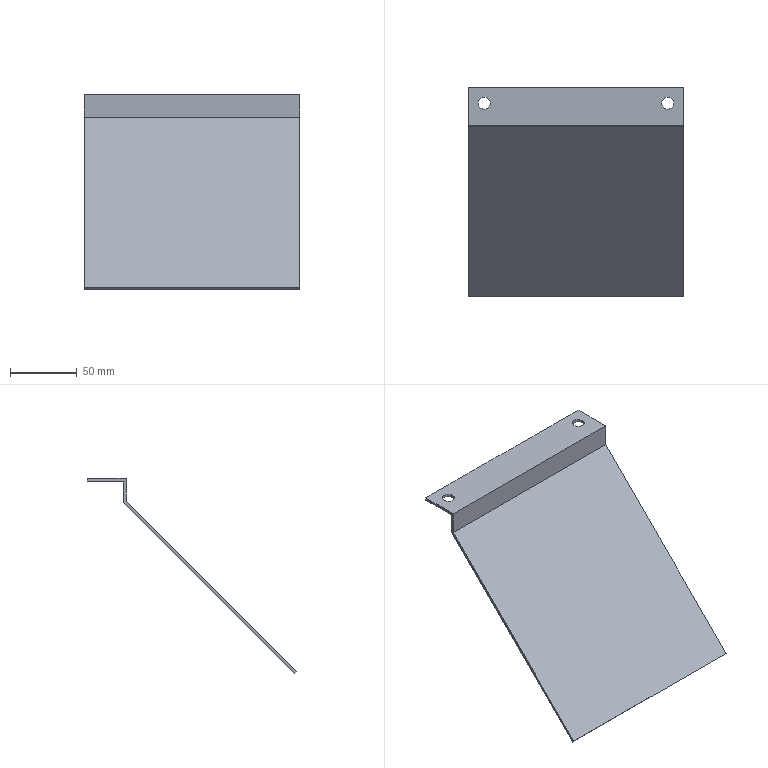Part | STEP file | lll_id4358_x_t | 1 solid | 12 faces | box 161.869 x 157.279 x 146.693 mm | volume 73016 mm3 | plane 10 | cylinder 2 | commonest cylinder face diameters 9 x2
STEP:
#1=CARTESIAN_POINT('',(1255.459,232.307,-325.279));
#2=VERTEX_POINT('',#1);
#3=CARTESIAN_POINT('',(1255.459,233.721,-326.693));
#4=VERTEX_POINT('',#3);
#5=CARTESIAN_POINT('',(1255.459,232.307,-325.279));
#6=DIRECTION('',(0.,0.7071,-0.7071));
#7=VECTOR('',#6,1.);
#8=LINE('',#5,#7);
#9=EDGE_CURVE('',#2,#4,#8,.T.);
#10=ORIENTED_EDGE('',*,*,#9,.T.);
#11=CARTESIAN_POINT('',(1417.328,233.721,-326.693));
#12=VERTEX_POINT('',#11);
#13=CARTESIAN_POINT('',(1417.328,233.721,-326.693));
#14=DIRECTION('',(-1.,0.,0.));
#15=VECTOR('',#14,1.);
#16=LINE('',#13,#15);
#17=EDGE_CURVE('',#12,#4,#16,.T.);
#18=ORIENTED_EDGE('',*,*,#17,.F.);
#19=CARTESIAN_POINT('',(1417.328,232.307,-325.279));
#20=VERTEX_POINT('',#19);
#21=CARTESIAN_POINT('',(1417.328,232.307,-325.279));
#22=DIRECTION('',(0.,0.7071,-0.7071));
#23=VECTOR('',#22,1.);
#24=LINE('',#21,#23);
#25=EDGE_CURVE('',#20,#12,#24,.T.);
#26=ORIENTED_EDGE('',*,*,#25,.F.);
#27=CARTESIAN_POINT('',(1417.328,232.307,-325.279));
#28=DIRECTION('',(-1.,0.,0.));
#29=VECTOR('',#28,1.);
#30=LINE('',#27,#29);
#31=EDGE_CURVE('',#20,#2,#30,.T.);
#32=ORIENTED_EDGE('',*,*,#31,.T.);
#33=EDGE_LOOP('',(#10,#18,#26,#32));
#34=FACE_OUTER_BOUND('',#33,.T.);
#35=CARTESIAN_POINT('',(1417.328,232.307,-325.279));
#36=DIRECTION('',(0.,-0.7071,-0.7071));
#37=DIRECTION('',(-1.,0.,0.));
#38=AXIS2_PLACEMENT_3D('',#35,#36,#37);
#39=PLANE('',#38);
#40=ADVANCED_FACE('',(#34),#39,.T.);
#41=CARTESIAN_POINT('',(1417.328,360.382,-197.204));
#42=VERTEX_POINT('',#41);
#43=CARTESIAN_POINT('',(1417.328,246.449,-311.137));
#44=DIRECTION('',(0.,-0.7071,-0.7071));
#45=VECTOR('',#44,1.);
#46=LINE('',#43,#45);
#47=EDGE_CURVE('',#42,#20,#46,.T.);
#48=ORIENTED_EDGE('',*,*,#47,.T.);
#49=ORIENTED_EDGE('',*,*,#25,.T.);
#50=CARTESIAN_POINT('',(1417.328,362.38,-198.034));
#51=VERTEX_POINT('',#50);
#52=CARTESIAN_POINT('',(1417.328,247.863,-312.551));
#53=DIRECTION('',(0.,-0.7071,-0.7071));
#54=VECTOR('',#53,1.);
#55=LINE('',#52,#54);
#56=EDGE_CURVE('',#51,#12,#55,.T.);
#57=ORIENTED_EDGE('',*,*,#56,.F.);
#58=CARTESIAN_POINT('',(1417.328,362.414,-182.));
#59=VERTEX_POINT('',#58);
#60=CARTESIAN_POINT('',(1417.328,362.414,-182.004));
#61=DIRECTION('',(0.,-0.00212,-1.));
#62=VECTOR('',#61,1.);
#63=LINE('',#60,#62);
#64=EDGE_CURVE('',#59,#51,#63,.T.);
#65=ORIENTED_EDGE('',*,*,#64,.F.);
#66=CARTESIAN_POINT('',(1417.328,389.586,-182.));
#67=VERTEX_POINT('',#66);
#68=CARTESIAN_POINT('',(1417.328,359.586,-182.));
#69=DIRECTION('',(0.,1.,0.));
#70=VECTOR('',#69,1.);
#71=LINE('',#68,#70);
#72=EDGE_CURVE('',#59,#67,#71,.T.);
#73=ORIENTED_EDGE('',*,*,#72,.T.);
#74=CARTESIAN_POINT('',(1417.328,389.586,-180.));
#75=VERTEX_POINT('',#74);
#76=CARTESIAN_POINT('',(1417.328,389.586,-293.137));
#77=DIRECTION('',(0.,0.,-1.));
#78=VECTOR('',#77,1.);
#79=LINE('',#76,#78);
#80=EDGE_CURVE('',#75,#67,#79,.T.);
#81=ORIENTED_EDGE('',*,*,#80,.F.);
#82=CARTESIAN_POINT('',(1417.328,360.418,-180.));
#83=VERTEX_POINT('',#82);
#84=CARTESIAN_POINT('',(1417.328,359.586,-180.));
#85=DIRECTION('',(0.,1.,0.));
#86=VECTOR('',#85,1.);
#87=LINE('',#84,#86);
#88=EDGE_CURVE('',#83,#75,#87,.T.);
#89=ORIENTED_EDGE('',*,*,#88,.F.);
#90=CARTESIAN_POINT('',(1417.328,360.178,-293.378));
#91=DIRECTION('',(0.,-0.00212,-1.));
#92=VECTOR('',#91,1.);
#93=LINE('',#90,#92);
#94=EDGE_CURVE('',#83,#42,#93,.T.);
#95=ORIENTED_EDGE('',*,*,#94,.T.);
#96=EDGE_LOOP('',(#48,#49,#57,#65,#73,#81,#89,#95));
#97=FACE_OUTER_BOUND('',#96,.T.);
#98=CARTESIAN_POINT('',(1417.328,246.449,-311.137));
#99=DIRECTION('',(-1.,0.,0.));
#100=DIRECTION('',(0.,0.7071,0.7071));
#101=AXIS2_PLACEMENT_3D('',#98,#99,#100);
#102=PLANE('',#101);
#103=ADVANCED_FACE('',(#97),#102,.F.);
#104=CARTESIAN_POINT('',(1255.459,362.38,-198.034));
#105=VERTEX_POINT('',#104);
#106=CARTESIAN_POINT('',(1255.459,247.863,-312.551));
#107=DIRECTION('',(0.,0.7071,0.7071));
#108=VECTOR('',#107,1.);
#109=LINE('',#106,#108);
#110=EDGE_CURVE('',#4,#105,#109,.T.);
#111=ORIENTED_EDGE('',*,*,#110,.F.);
#112=ORIENTED_EDGE('',*,*,#9,.F.);
#113=CARTESIAN_POINT('',(1255.459,360.382,-197.204));
#114=VERTEX_POINT('',#113);
#115=CARTESIAN_POINT('',(1255.459,246.449,-311.137));
#116=DIRECTION('',(0.,0.7071,0.7071));
#117=VECTOR('',#116,1.);
#118=LINE('',#115,#117);
#119=EDGE_CURVE('',#2,#114,#118,.T.);
#120=ORIENTED_EDGE('',*,*,#119,.T.);
#121=CARTESIAN_POINT('',(1255.459,360.418,-180.));
#122=VERTEX_POINT('',#121);
#123=CARTESIAN_POINT('',(1255.459,360.178,-293.378));
#124=DIRECTION('',(0.,-0.00212,-1.));
#125=VECTOR('',#124,1.);
#126=LINE('',#123,#125);
#127=EDGE_CURVE('',#122,#114,#126,.T.);
#128=ORIENTED_EDGE('',*,*,#127,.F.);
#129=CARTESIAN_POINT('',(1255.459,389.586,-180.));
#130=VERTEX_POINT('',#129);
#131=CARTESIAN_POINT('',(1255.459,359.586,-180.));
#132=DIRECTION('',(0.,-1.,0.));
#133=VECTOR('',#132,1.);
#134=LINE('',#131,#133);
#135=EDGE_CURVE('',#130,#122,#134,.T.);
#136=ORIENTED_EDGE('',*,*,#135,.F.);
#137=CARTESIAN_POINT('',(1255.459,389.586,-182.));
#138=VERTEX_POINT('',#137);
#139=CARTESIAN_POINT('',(1255.459,389.586,-180.));
#140=DIRECTION('',(0.,0.,-1.));
#141=VECTOR('',#140,1.);
#142=LINE('',#139,#141);
#143=EDGE_CURVE('',#130,#138,#142,.T.);
#144=ORIENTED_EDGE('',*,*,#143,.T.);
#145=CARTESIAN_POINT('',(1255.459,362.414,-182.));
#146=VERTEX_POINT('',#145);
#147=CARTESIAN_POINT('',(1255.459,359.586,-182.));
#148=DIRECTION('',(0.,-1.,0.));
#149=VECTOR('',#148,1.);
#150=LINE('',#147,#149);
#151=EDGE_CURVE('',#138,#146,#150,.T.);
#152=ORIENTED_EDGE('',*,*,#151,.T.);
#153=CARTESIAN_POINT('',(1255.459,362.414,-182.004));
#154=DIRECTION('',(0.,-0.00212,-1.));
#155=VECTOR('',#154,1.);
#156=LINE('',#153,#155);
#157=EDGE_CURVE('',#146,#105,#156,.T.);
#158=ORIENTED_EDGE('',*,*,#157,.T.);
#159=EDGE_LOOP('',(#111,#112,#120,#128,#136,#144,#152,#158));
#160=FACE_OUTER_BOUND('',#159,.T.);
#161=CARTESIAN_POINT('',(1255.459,246.449,-311.137));
#162=DIRECTION('',(-1.,0.,0.));
#163=DIRECTION('',(0.,0.7071,0.7071));
#164=AXIS2_PLACEMENT_3D('',#161,#162,#163);
#165=PLANE('',#164);
#166=ADVANCED_FACE('',(#160),#165,.T.);
#167=ORIENTED_EDGE('',*,*,#56,.T.);
#168=ORIENTED_EDGE('',*,*,#17,.T.);
#169=ORIENTED_EDGE('',*,*,#110,.T.);
#170=CARTESIAN_POINT('',(-1607.432,362.38,-198.034));
#171=DIRECTION('',(-1.,0.,0.));
#172=VECTOR('',#171,1.);
#173=LINE('',#170,#172);
#174=EDGE_CURVE('',#51,#105,#173,.T.);
#175=ORIENTED_EDGE('',*,*,#174,.F.);
#176=EDGE_LOOP('',(#167,#168,#169,#175));
#177=FACE_OUTER_BOUND('',#176,.T.);
#178=CARTESIAN_POINT('',(1417.328,247.863,-312.551));
#179=DIRECTION('',(0.,-0.7071,0.7071));
#180=DIRECTION('',(0.,0.7071,0.7071));
#181=AXIS2_PLACEMENT_3D('',#178,#179,#180);
#182=PLANE('',#181);
#183=ADVANCED_FACE('',(#177),#182,.F.);
#184=CARTESIAN_POINT('',(1417.328,360.382,-197.204));
#185=DIRECTION('',(-1.,0.,0.));
#186=VECTOR('',#185,1.);
#187=LINE('',#184,#186);
#188=EDGE_CURVE('',#42,#114,#187,.T.);
#189=ORIENTED_EDGE('',*,*,#188,.T.);
#190=ORIENTED_EDGE('',*,*,#119,.F.);
#191=ORIENTED_EDGE('',*,*,#31,.F.);
#192=ORIENTED_EDGE('',*,*,#47,.F.);
#193=EDGE_LOOP('',(#189,#190,#191,#192));
#194=FACE_OUTER_BOUND('',#193,.T.);
#195=CARTESIAN_POINT('',(1417.328,246.449,-311.137));
#196=DIRECTION('',(0.,-0.7071,0.7071));
#197=DIRECTION('',(0.,0.7071,0.7071));
#198=AXIS2_PLACEMENT_3D('',#195,#196,#197);
#199=PLANE('',#198);
#200=ADVANCED_FACE('',(#194),#199,.T.);
#201=ORIENTED_EDGE('',*,*,#64,.T.);
#202=ORIENTED_EDGE('',*,*,#174,.T.);
#203=ORIENTED_EDGE('',*,*,#157,.F.);
#204=CARTESIAN_POINT('',(-1607.432,362.414,-182.));
#205=DIRECTION('',(-1.,0.,0.));
#206=VECTOR('',#205,1.);
#207=LINE('',#204,#206);
#208=EDGE_CURVE('',#59,#146,#207,.T.);
#209=ORIENTED_EDGE('',*,*,#208,.F.);
#210=EDGE_LOOP('',(#201,#202,#203,#209));
#211=FACE_OUTER_BOUND('',#210,.T.);
#212=CARTESIAN_POINT('',(-1607.432,362.414,-182.004));
#213=DIRECTION('',(0.,-1.,0.00212));
#214=DIRECTION('',(0.,0.00212,1.));
#215=AXIS2_PLACEMENT_3D('',#212,#213,#214);
#216=PLANE('',#215);
#217=ADVANCED_FACE('',(#211),#216,.F.);
#218=ORIENTED_EDGE('',*,*,#94,.F.);
#219=CARTESIAN_POINT('',(1275.459,360.418,-180.));
#220=DIRECTION('',(1.,0.,0.));
#221=VECTOR('',#220,1.);
#222=LINE('',#219,#221);
#223=EDGE_CURVE('',#122,#83,#222,.T.);
#224=ORIENTED_EDGE('',*,*,#223,.F.);
#225=ORIENTED_EDGE('',*,*,#127,.T.);
#226=ORIENTED_EDGE('',*,*,#188,.F.);
#227=EDGE_LOOP('',(#218,#224,#225,#226));
#228=FACE_OUTER_BOUND('',#227,.T.);
#229=CARTESIAN_POINT('',(-1607.432,360.414,-182.));
#230=DIRECTION('',(0.,-1.,0.00212));
#231=DIRECTION('',(0.,0.00212,1.));
#232=AXIS2_PLACEMENT_3D('',#229,#230,#231);
#233=PLANE('',#232);
#234=ADVANCED_FACE('',(#228),#233,.T.);
#235=CARTESIAN_POINT('',(1409.828,377.586,-182.));
#236=VERTEX_POINT('',#235);
#237=CARTESIAN_POINT('',(1405.328,377.586,-182.));
#238=DIRECTION('',(0.,0.,-1.));
#239=DIRECTION('',(1.,0.,0.));
#240=AXIS2_PLACEMENT_3D('',#237,#238,#239);
#241=CIRCLE('',#240,4.5);
#242=EDGE_CURVE('',#236,#236,#241,.T.);
#243=ORIENTED_EDGE('',*,*,#242,.F.);
#244=EDGE_LOOP('',(#243));
#245=FACE_BOUND('',#244,.T.);
#246=CARTESIAN_POINT('',(1271.959,377.586,-182.));
#247=VERTEX_POINT('',#246);
#248=CARTESIAN_POINT('',(1267.459,377.586,-182.));
#249=DIRECTION('',(0.,0.,-1.));
#250=DIRECTION('',(1.,0.,0.));
#251=AXIS2_PLACEMENT_3D('',#248,#249,#250);
#252=CIRCLE('',#251,4.5);
#253=EDGE_CURVE('',#247,#247,#252,.T.);
#254=ORIENTED_EDGE('',*,*,#253,.F.);
#255=EDGE_LOOP('',(#254));
#256=FACE_BOUND('',#255,.T.);
#257=ORIENTED_EDGE('',*,*,#208,.T.);
#258=ORIENTED_EDGE('',*,*,#151,.F.);
#259=CARTESIAN_POINT('',(1275.459,389.586,-182.));
#260=DIRECTION('',(-1.,0.,0.));
#261=VECTOR('',#260,1.);
#262=LINE('',#259,#261);
#263=EDGE_CURVE('',#67,#138,#262,.T.);
#264=ORIENTED_EDGE('',*,*,#263,.F.);
#265=ORIENTED_EDGE('',*,*,#72,.F.);
#266=EDGE_LOOP('',(#257,#258,#264,#265));
#267=FACE_BOUND('',#266,.T.);
#268=CARTESIAN_POINT('',(1275.459,359.586,-182.));
#269=DIRECTION('',(0.,0.,-1.));
#270=DIRECTION('',(-1.,0.,0.));
#271=AXIS2_PLACEMENT_3D('',#268,#269,#270);
#272=PLANE('',#271);
#273=ADVANCED_FACE('',(#245,#256,#267),#272,.T.);
#274=ORIENTED_EDGE('',*,*,#80,.T.);
#275=ORIENTED_EDGE('',*,*,#263,.T.);
#276=ORIENTED_EDGE('',*,*,#143,.F.);
#277=CARTESIAN_POINT('',(1275.459,389.586,-180.));
#278=DIRECTION('',(-1.,0.,0.));
#279=VECTOR('',#278,1.);
#280=LINE('',#277,#279);
#281=EDGE_CURVE('',#75,#130,#280,.T.);
#282=ORIENTED_EDGE('',*,*,#281,.F.);
#283=EDGE_LOOP('',(#274,#275,#276,#282));
#284=FACE_OUTER_BOUND('',#283,.T.);
#285=CARTESIAN_POINT('',(1275.459,389.586,-180.));
#286=DIRECTION('',(0.,-1.,0.));
#287=DIRECTION('',(1.,0.,0.));
#288=AXIS2_PLACEMENT_3D('',#285,#286,#287);
#289=PLANE('',#288);
#290=ADVANCED_FACE('',(#284),#289,.F.);
#291=ORIENTED_EDGE('',*,*,#253,.T.);
#292=EDGE_LOOP('',(#291));
#293=FACE_BOUND('',#292,.T.);
#294=CARTESIAN_POINT('',(1262.959,377.586,-180.));
#295=VERTEX_POINT('',#294);
#296=CARTESIAN_POINT('',(1267.459,377.586,-180.));
#297=DIRECTION('',(0.,0.,1.));
#298=DIRECTION('',(-1.,0.,0.));
#299=AXIS2_PLACEMENT_3D('',#296,#297,#298);
#300=CIRCLE('',#299,4.5);
#301=EDGE_CURVE('',#295,#295,#300,.T.);
#302=ORIENTED_EDGE('',*,*,#301,.T.);
#303=EDGE_LOOP('',(#302));
#304=FACE_BOUND('',#303,.T.);
#305=CARTESIAN_POINT('',(1267.459,377.586,-182.));
#306=DIRECTION('',(0.,0.,1.));
#307=DIRECTION('',(1.,0.,0.));
#308=AXIS2_PLACEMENT_3D('',#305,#306,#307);
#309=CYLINDRICAL_SURFACE('',#308,4.5);
#310=ADVANCED_FACE('',(#293,#304),#309,.F.);
#311=ORIENTED_EDGE('',*,*,#242,.T.);
#312=EDGE_LOOP('',(#311));
#313=FACE_BOUND('',#312,.T.);
#314=CARTESIAN_POINT('',(1400.828,377.586,-180.));
#315=VERTEX_POINT('',#314);
#316=CARTESIAN_POINT('',(1405.328,377.586,-180.));
#317=DIRECTION('',(0.,0.,1.));
#318=DIRECTION('',(-1.,0.,0.));
#319=AXIS2_PLACEMENT_3D('',#316,#317,#318);
#320=CIRCLE('',#319,4.5);
#321=EDGE_CURVE('',#315,#315,#320,.T.);
#322=ORIENTED_EDGE('',*,*,#321,.T.);
#323=EDGE_LOOP('',(#322));
#324=FACE_BOUND('',#323,.T.);
#325=CARTESIAN_POINT('',(1405.328,377.586,-182.));
#326=DIRECTION('',(0.,0.,1.));
#327=DIRECTION('',(1.,0.,0.));
#328=AXIS2_PLACEMENT_3D('',#325,#326,#327);
#329=CYLINDRICAL_SURFACE('',#328,4.5);
#330=ADVANCED_FACE('',(#313,#324),#329,.F.);
#331=ORIENTED_EDGE('',*,*,#321,.F.);
#332=EDGE_LOOP('',(#331));
#333=FACE_BOUND('',#332,.T.);
#334=ORIENTED_EDGE('',*,*,#301,.F.);
#335=EDGE_LOOP('',(#334));
#336=FACE_BOUND('',#335,.T.);
#337=ORIENTED_EDGE('',*,*,#223,.T.);
#338=ORIENTED_EDGE('',*,*,#88,.T.);
#339=ORIENTED_EDGE('',*,*,#281,.T.);
#340=ORIENTED_EDGE('',*,*,#135,.T.);
#341=EDGE_LOOP('',(#337,#338,#339,#340));
#342=FACE_BOUND('',#341,.T.);
#343=CARTESIAN_POINT('',(1275.459,359.586,-180.));
#344=DIRECTION('',(0.,0.,-1.));
#345=DIRECTION('',(-1.,0.,0.));
#346=AXIS2_PLACEMENT_3D('',#343,#344,#345);
#347=PLANE('',#346);
#348=ADVANCED_FACE('',(#333,#336,#342),#347,.F.);
#349=CLOSED_SHELL('',(#40,#103,#166,#183,#200,#217,#234,#273,#290,#310,#330,#348));
#350=MANIFOLD_SOLID_BREP('',#349);
#351=(LENGTH_UNIT()NAMED_UNIT(*)SI_UNIT(.MILLI.,.METRE.));
#352=UNCERTAINTY_MEASURE_WITH_UNIT(LENGTH_MEASURE(0.00002),#351,'','');
#353=(NAMED_UNIT(*)PLANE_ANGLE_UNIT()SI_UNIT($,.RADIAN.));
#354=PLANE_ANGLE_MEASURE_WITH_UNIT(PLANE_ANGLE_MEASURE(0.01745),#353);
#355=DIMENSIONAL_EXPONENTS(0.,0.,0.,0.,0.,0.,0.);
#356=(CONVERSION_BASED_UNIT('DEGREE',#354)NAMED_UNIT(#355)PLANE_ANGLE_UNIT());
#357=(NAMED_UNIT(*)SI_UNIT($,.STERADIAN.)SOLID_ANGLE_UNIT());
#358=(GEOMETRIC_REPRESENTATION_CONTEXT(3)GLOBAL_UNCERTAINTY_ASSIGNED_CONTEXT((#352))GLOBAL_UNIT_ASSIGNED_CONTEXT((#351,#356,#357))REPRESENTATION_CONTEXT('',''));
#359=ADVANCED_BREP_SHAPE_REPRESENTATION('',(#350),#358);